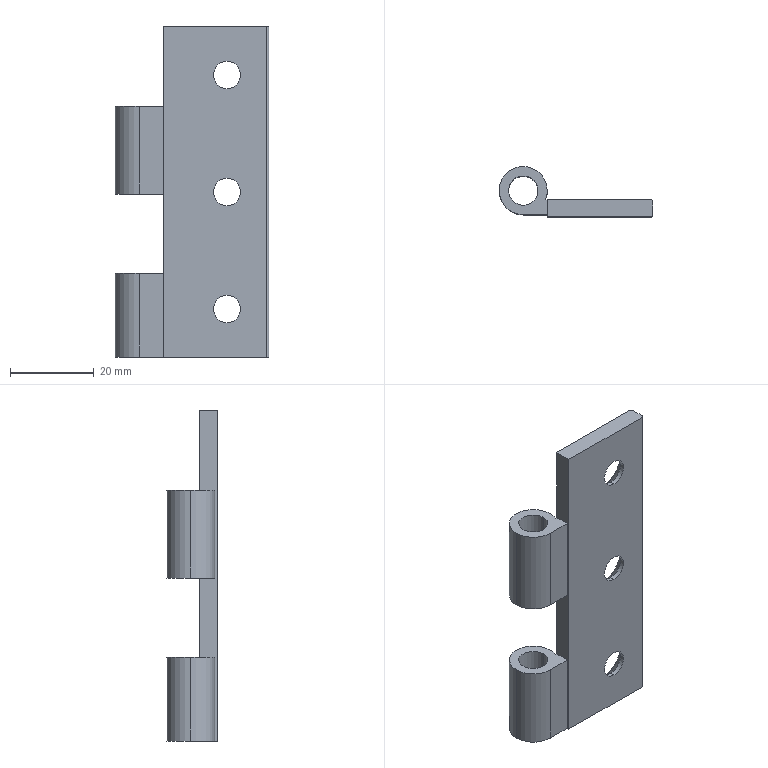Part | SolidWorks | features BaseBody 1 | 1 solid | 35 faces | box 36.75 x 12.05 x 79 mm | volume 10360 mm3 | cylinder 18 | plane 11 | cone 6 | commonest cylinder face diameters 6.5 x6 11.5 x6 7 x4 1 x2
STEP:
#1=CARTESIAN_POINT('',(21.,0.,-24.75));
#2=VERTEX_POINT('',#1);
#3=CARTESIAN_POINT('',(21.,0.,-31.25));
#4=VERTEX_POINT('',#3);
#5=CARTESIAN_POINT('',(21.,0.,-28.));
#6=DIRECTION('',(0.,-1.,0.));
#7=DIRECTION('',(0.,0.,1.));
#8=AXIS2_PLACEMENT_3D('',#5,#6,#7);
#9=CIRCLE('',#8,3.25);
#10=EDGE_CURVE('',#2,#4,#9,.T.);
#11=ORIENTED_EDGE('',*,*,#10,.T.);
#12=CARTESIAN_POINT('',(21.,1.1,-31.25));
#13=VERTEX_POINT('',#12);
#14=CARTESIAN_POINT('',(21.,0.,-31.25));
#15=DIRECTION('',(0.,1.,0.));
#16=VECTOR('',#15,1000.);
#17=LINE('',#14,#16);
#18=EDGE_CURVE('',#4,#13,#17,.T.);
#19=ORIENTED_EDGE('',*,*,#18,.T.);
#20=CARTESIAN_POINT('',(21.,1.1,-24.75));
#21=VERTEX_POINT('',#20);
#22=CARTESIAN_POINT('',(21.,1.1,-28.));
#23=DIRECTION('',(0.,-1.,0.));
#24=DIRECTION('',(0.,0.,1.));
#25=AXIS2_PLACEMENT_3D('',#22,#23,#24);
#26=CIRCLE('',#25,3.25);
#27=EDGE_CURVE('',#21,#13,#26,.T.);
#28=ORIENTED_EDGE('',*,*,#27,.F.);
#29=CARTESIAN_POINT('',(21.,0.,-24.75));
#30=DIRECTION('',(0.,1.,0.));
#31=VECTOR('',#30,1000.);
#32=LINE('',#29,#31);
#33=EDGE_CURVE('',#2,#21,#32,.T.);
#34=ORIENTED_EDGE('',*,*,#33,.F.);
#35=EDGE_LOOP('',(#11,#19,#28,#34));
#36=FACE_OUTER_BOUND('',#35,.T.);
#37=CARTESIAN_POINT('',(21.,0.,-28.));
#38=DIRECTION('',(0.,1.,0.));
#39=DIRECTION('',(0.,0.,1.));
#40=AXIS2_PLACEMENT_3D('',#37,#38,#39);
#41=CYLINDRICAL_SURFACE('',#40,3.25);
#42=ADVANCED_FACE('',(#36),#41,.F.);
#43=CARTESIAN_POINT('',(21.,0.,3.25));
#44=VERTEX_POINT('',#43);
#45=CARTESIAN_POINT('',(21.,0.,-3.25));
#46=VERTEX_POINT('',#45);
#47=CARTESIAN_POINT('',(21.,0.,0.));
#48=DIRECTION('',(0.,-1.,0.));
#49=DIRECTION('',(0.,0.,1.));
#50=AXIS2_PLACEMENT_3D('',#47,#48,#49);
#51=CIRCLE('',#50,3.25);
#52=EDGE_CURVE('',#44,#46,#51,.T.);
#53=ORIENTED_EDGE('',*,*,#52,.T.);
#54=CARTESIAN_POINT('',(21.,1.1,-3.25));
#55=VERTEX_POINT('',#54);
#56=CARTESIAN_POINT('',(21.,0.,-3.25));
#57=DIRECTION('',(0.,1.,0.));
#58=VECTOR('',#57,1000.);
#59=LINE('',#56,#58);
#60=EDGE_CURVE('',#46,#55,#59,.T.);
#61=ORIENTED_EDGE('',*,*,#60,.T.);
#62=CARTESIAN_POINT('',(21.,1.1,3.25));
#63=VERTEX_POINT('',#62);
#64=CARTESIAN_POINT('',(21.,1.1,0.));
#65=DIRECTION('',(0.,-1.,0.));
#66=DIRECTION('',(0.,0.,1.));
#67=AXIS2_PLACEMENT_3D('',#64,#65,#66);
#68=CIRCLE('',#67,3.25);
#69=EDGE_CURVE('',#63,#55,#68,.T.);
#70=ORIENTED_EDGE('',*,*,#69,.F.);
#71=CARTESIAN_POINT('',(21.,0.,3.25));
#72=DIRECTION('',(0.,1.,0.));
#73=VECTOR('',#72,1000.);
#74=LINE('',#71,#73);
#75=EDGE_CURVE('',#44,#63,#74,.T.);
#76=ORIENTED_EDGE('',*,*,#75,.F.);
#77=EDGE_LOOP('',(#53,#61,#70,#76));
#78=FACE_OUTER_BOUND('',#77,.T.);
#79=CARTESIAN_POINT('',(21.,0.,0.));
#80=DIRECTION('',(0.,1.,0.));
#81=DIRECTION('',(0.,0.,1.));
#82=AXIS2_PLACEMENT_3D('',#79,#80,#81);
#83=CYLINDRICAL_SURFACE('',#82,3.25);
#84=ADVANCED_FACE('',(#78),#83,.F.);
#85=CARTESIAN_POINT('',(21.,0.,31.25));
#86=VERTEX_POINT('',#85);
#87=CARTESIAN_POINT('',(21.,0.,24.75));
#88=VERTEX_POINT('',#87);
#89=CARTESIAN_POINT('',(21.,0.,28.));
#90=DIRECTION('',(0.,-1.,0.));
#91=DIRECTION('',(0.,0.,1.));
#92=AXIS2_PLACEMENT_3D('',#89,#90,#91);
#93=CIRCLE('',#92,3.25);
#94=EDGE_CURVE('',#86,#88,#93,.T.);
#95=ORIENTED_EDGE('',*,*,#94,.T.);
#96=CARTESIAN_POINT('',(21.,1.1,24.75));
#97=VERTEX_POINT('',#96);
#98=CARTESIAN_POINT('',(21.,0.,24.75));
#99=DIRECTION('',(0.,1.,0.));
#100=VECTOR('',#99,1000.);
#101=LINE('',#98,#100);
#102=EDGE_CURVE('',#88,#97,#101,.T.);
#103=ORIENTED_EDGE('',*,*,#102,.T.);
#104=CARTESIAN_POINT('',(21.,1.1,31.25));
#105=VERTEX_POINT('',#104);
#106=CARTESIAN_POINT('',(21.,1.1,28.));
#107=DIRECTION('',(0.,-1.,0.));
#108=DIRECTION('',(0.,0.,1.));
#109=AXIS2_PLACEMENT_3D('',#106,#107,#108);
#110=CIRCLE('',#109,3.25);
#111=EDGE_CURVE('',#105,#97,#110,.T.);
#112=ORIENTED_EDGE('',*,*,#111,.F.);
#113=CARTESIAN_POINT('',(21.,0.,31.25));
#114=DIRECTION('',(0.,1.,0.));
#115=VECTOR('',#114,1000.);
#116=LINE('',#113,#115);
#117=EDGE_CURVE('',#86,#105,#116,.T.);
#118=ORIENTED_EDGE('',*,*,#117,.F.);
#119=EDGE_LOOP('',(#95,#103,#112,#118));
#120=FACE_OUTER_BOUND('',#119,.T.);
#121=CARTESIAN_POINT('',(21.,0.,28.));
#122=DIRECTION('',(0.,1.,0.));
#123=DIRECTION('',(0.,0.,1.));
#124=AXIS2_PLACEMENT_3D('',#121,#122,#123);
#125=CYLINDRICAL_SURFACE('',#124,3.25);
#126=ADVANCED_FACE('',(#120),#125,.F.);
#127=CARTESIAN_POINT('',(5.75,6.3,-39.5));
#128=VERTEX_POINT('',#127);
#129=CARTESIAN_POINT('',(-5.75,6.3,-39.5));
#130=VERTEX_POINT('',#129);
#131=CARTESIAN_POINT('',(0.,6.3,-39.5));
#132=DIRECTION('',(0.,0.,1.));
#133=DIRECTION('',(1.,0.,0.));
#134=AXIS2_PLACEMENT_3D('',#131,#132,#133);
#135=CIRCLE('',#134,5.75);
#136=EDGE_CURVE('',#128,#130,#135,.T.);
#137=ORIENTED_EDGE('',*,*,#136,.T.);
#138=CARTESIAN_POINT('',(-5.75,6.3,-19.5));
#139=VERTEX_POINT('',#138);
#140=CARTESIAN_POINT('',(-5.75,6.3,39.5));
#141=DIRECTION('',(0.,0.,1.));
#142=VECTOR('',#141,1000.);
#143=LINE('',#140,#142);
#144=EDGE_CURVE('',#130,#139,#143,.T.);
#145=ORIENTED_EDGE('',*,*,#144,.T.);
#146=CARTESIAN_POINT('',(5.75,6.3,-19.5));
#147=VERTEX_POINT('',#146);
#148=CARTESIAN_POINT('',(0.,6.3,-19.5));
#149=DIRECTION('',(0.,0.,-1.));
#150=DIRECTION('',(1.,0.,0.));
#151=AXIS2_PLACEMENT_3D('',#148,#149,#150);
#152=CIRCLE('',#151,5.75);
#153=EDGE_CURVE('',#139,#147,#152,.T.);
#154=ORIENTED_EDGE('',*,*,#153,.T.);
#155=CARTESIAN_POINT('',(5.75,6.3,39.5));
#156=DIRECTION('',(0.,0.,1.));
#157=VECTOR('',#156,1000.);
#158=LINE('',#155,#157);
#159=EDGE_CURVE('',#128,#147,#158,.T.);
#160=ORIENTED_EDGE('',*,*,#159,.F.);
#161=EDGE_LOOP('',(#137,#145,#154,#160));
#162=FACE_OUTER_BOUND('',#161,.T.);
#163=CARTESIAN_POINT('',(0.,6.3,39.5));
#164=DIRECTION('',(0.,0.,1.));
#165=DIRECTION('',(1.,0.,0.));
#166=AXIS2_PLACEMENT_3D('',#163,#164,#165);
#167=CYLINDRICAL_SURFACE('',#166,5.75);
#168=ADVANCED_FACE('',(#162),#167,.T.);
#169=CARTESIAN_POINT('',(5.312,4.1,-39.5));
#170=VERTEX_POINT('',#169);
#171=CARTESIAN_POINT('',(0.,6.3,-39.5));
#172=DIRECTION('',(0.,0.,1.));
#173=DIRECTION('',(1.,0.,0.));
#174=AXIS2_PLACEMENT_3D('',#171,#172,#173);
#175=CIRCLE('',#174,5.75);
#176=EDGE_CURVE('',#170,#128,#175,.T.);
#177=ORIENTED_EDGE('',*,*,#176,.T.);
#178=ORIENTED_EDGE('',*,*,#159,.T.);
#179=CARTESIAN_POINT('',(5.312,4.1,-19.5));
#180=VERTEX_POINT('',#179);
#181=CARTESIAN_POINT('',(0.,6.3,-19.5));
#182=DIRECTION('',(0.,0.,-1.));
#183=DIRECTION('',(1.,0.,0.));
#184=AXIS2_PLACEMENT_3D('',#181,#182,#183);
#185=CIRCLE('',#184,5.75);
#186=EDGE_CURVE('',#147,#180,#185,.T.);
#187=ORIENTED_EDGE('',*,*,#186,.T.);
#188=CARTESIAN_POINT('',(5.312,4.1,39.5));
#189=DIRECTION('',(0.,0.,-1.));
#190=VECTOR('',#189,1000.);
#191=LINE('',#188,#190);
#192=EDGE_CURVE('',#180,#170,#191,.T.);
#193=ORIENTED_EDGE('',*,*,#192,.T.);
#194=EDGE_LOOP('',(#177,#178,#187,#193));
#195=FACE_OUTER_BOUND('',#194,.T.);
#196=CARTESIAN_POINT('',(0.,6.3,39.5));
#197=DIRECTION('',(0.,0.,1.));
#198=DIRECTION('',(1.,0.,0.));
#199=AXIS2_PLACEMENT_3D('',#196,#197,#198);
#200=CYLINDRICAL_SURFACE('',#199,5.75);
#201=ADVANCED_FACE('',(#195),#200,.T.);
#202=CARTESIAN_POINT('',(3.5,6.3,-39.5));
#203=VERTEX_POINT('',#202);
#204=CARTESIAN_POINT('',(-3.5,6.3,-39.5));
#205=VERTEX_POINT('',#204);
#206=CARTESIAN_POINT('',(0.,6.3,-39.5));
#207=DIRECTION('',(0.,0.,-1.));
#208=DIRECTION('',(1.,0.,0.));
#209=AXIS2_PLACEMENT_3D('',#206,#207,#208);
#210=CIRCLE('',#209,3.5);
#211=EDGE_CURVE('',#203,#205,#210,.T.);
#212=ORIENTED_EDGE('',*,*,#211,.T.);
#213=CARTESIAN_POINT('',(-3.5,6.3,-19.5));
#214=VERTEX_POINT('',#213);
#215=CARTESIAN_POINT('',(-3.5,6.3,39.5));
#216=DIRECTION('',(0.,0.,1.));
#217=VECTOR('',#216,1000.);
#218=LINE('',#215,#217);
#219=EDGE_CURVE('',#205,#214,#218,.T.);
#220=ORIENTED_EDGE('',*,*,#219,.T.);
#221=CARTESIAN_POINT('',(3.5,6.3,-19.5));
#222=VERTEX_POINT('',#221);
#223=CARTESIAN_POINT('',(0.,6.3,-19.5));
#224=DIRECTION('',(0.,0.,-1.));
#225=DIRECTION('',(1.,0.,0.));
#226=AXIS2_PLACEMENT_3D('',#223,#224,#225);
#227=CIRCLE('',#226,3.5);
#228=EDGE_CURVE('',#222,#214,#227,.T.);
#229=ORIENTED_EDGE('',*,*,#228,.F.);
#230=CARTESIAN_POINT('',(3.5,6.3,39.5));
#231=DIRECTION('',(0.,0.,1.));
#232=VECTOR('',#231,1000.);
#233=LINE('',#230,#232);
#234=EDGE_CURVE('',#203,#222,#233,.T.);
#235=ORIENTED_EDGE('',*,*,#234,.F.);
#236=EDGE_LOOP('',(#212,#220,#229,#235));
#237=FACE_OUTER_BOUND('',#236,.T.);
#238=CARTESIAN_POINT('',(0.,6.3,39.5));
#239=DIRECTION('',(0.,0.,1.));
#240=DIRECTION('',(1.,0.,0.));
#241=AXIS2_PLACEMENT_3D('',#238,#239,#240);
#242=CYLINDRICAL_SURFACE('',#241,3.5);
#243=ADVANCED_FACE('',(#237),#242,.F.);
#244=ORIENTED_EDGE('',*,*,#27,.T.);
#245=CARTESIAN_POINT('',(21.,4.1,-34.25));
#246=VERTEX_POINT('',#245);
#247=CARTESIAN_POINT('',(21.,4.1,-34.25));
#248=DIRECTION('',(0.,0.7071,-0.7071));
#249=VECTOR('',#248,1000.);
#250=LINE('',#247,#249);
#251=EDGE_CURVE('',#13,#246,#250,.T.);
#252=ORIENTED_EDGE('',*,*,#251,.T.);
#253=CARTESIAN_POINT('',(21.,4.1,-21.75));
#254=VERTEX_POINT('',#253);
#255=CARTESIAN_POINT('',(21.,4.1,-28.));
#256=DIRECTION('',(0.,1.,0.));
#257=DIRECTION('',(0.,0.,1.));
#258=AXIS2_PLACEMENT_3D('',#255,#256,#257);
#259=CIRCLE('',#258,6.25);
#260=EDGE_CURVE('',#246,#254,#259,.T.);
#261=ORIENTED_EDGE('',*,*,#260,.T.);
#262=CARTESIAN_POINT('',(21.,4.1,-21.75));
#263=DIRECTION('',(0.,0.7071,0.7071));
#264=VECTOR('',#263,1000.);
#265=LINE('',#262,#264);
#266=EDGE_CURVE('',#21,#254,#265,.T.);
#267=ORIENTED_EDGE('',*,*,#266,.F.);
#268=EDGE_LOOP('',(#244,#252,#261,#267));
#269=FACE_OUTER_BOUND('',#268,.T.);
#270=CARTESIAN_POINT('',(21.,4.1,-28.));
#271=DIRECTION('',(0.,1.,0.));
#272=DIRECTION('',(0.,0.,1.));
#273=AXIS2_PLACEMENT_3D('',#270,#271,#272);
#274=CONICAL_SURFACE('',#273,6.25,0.7854);
#275=ADVANCED_FACE('',(#269),#274,.F.);
#276=ORIENTED_EDGE('',*,*,#69,.T.);
#277=CARTESIAN_POINT('',(21.,4.1,-6.25));
#278=VERTEX_POINT('',#277);
#279=CARTESIAN_POINT('',(21.,4.1,-6.25));
#280=DIRECTION('',(0.,0.7071,-0.7071));
#281=VECTOR('',#280,1000.);
#282=LINE('',#279,#281);
#283=EDGE_CURVE('',#55,#278,#282,.T.);
#284=ORIENTED_EDGE('',*,*,#283,.T.);
#285=CARTESIAN_POINT('',(21.,4.1,6.25));
#286=VERTEX_POINT('',#285);
#287=CARTESIAN_POINT('',(21.,4.1,0.));
#288=DIRECTION('',(0.,1.,0.));
#289=DIRECTION('',(0.,0.,1.));
#290=AXIS2_PLACEMENT_3D('',#287,#288,#289);
#291=CIRCLE('',#290,6.25);
#292=EDGE_CURVE('',#278,#286,#291,.T.);
#293=ORIENTED_EDGE('',*,*,#292,.T.);
#294=CARTESIAN_POINT('',(21.,4.1,6.25));
#295=DIRECTION('',(0.,0.7071,0.7071));
#296=VECTOR('',#295,1000.);
#297=LINE('',#294,#296);
#298=EDGE_CURVE('',#63,#286,#297,.T.);
#299=ORIENTED_EDGE('',*,*,#298,.F.);
#300=EDGE_LOOP('',(#276,#284,#293,#299));
#301=FACE_OUTER_BOUND('',#300,.T.);
#302=CARTESIAN_POINT('',(21.,4.1,0.));
#303=DIRECTION('',(0.,1.,0.));
#304=DIRECTION('',(0.,0.,1.));
#305=AXIS2_PLACEMENT_3D('',#302,#303,#304);
#306=CONICAL_SURFACE('',#305,6.25,0.7854);
#307=ADVANCED_FACE('',(#301),#306,.F.);
#308=ORIENTED_EDGE('',*,*,#111,.T.);
#309=CARTESIAN_POINT('',(21.,4.1,21.75));
#310=VERTEX_POINT('',#309);
#311=CARTESIAN_POINT('',(21.,4.1,21.75));
#312=DIRECTION('',(0.,0.7071,-0.7071));
#313=VECTOR('',#312,1000.);
#314=LINE('',#311,#313);
#315=EDGE_CURVE('',#97,#310,#314,.T.);
#316=ORIENTED_EDGE('',*,*,#315,.T.);
#317=CARTESIAN_POINT('',(21.,4.1,34.25));
#318=VERTEX_POINT('',#317);
#319=CARTESIAN_POINT('',(21.,4.1,28.));
#320=DIRECTION('',(0.,1.,0.));
#321=DIRECTION('',(0.,0.,1.));
#322=AXIS2_PLACEMENT_3D('',#319,#320,#321);
#323=CIRCLE('',#322,6.25);
#324=EDGE_CURVE('',#310,#318,#323,.T.);
#325=ORIENTED_EDGE('',*,*,#324,.T.);
#326=CARTESIAN_POINT('',(21.,4.1,34.25));
#327=DIRECTION('',(0.,0.7071,0.7071));
#328=VECTOR('',#327,1000.);
#329=LINE('',#326,#328);
#330=EDGE_CURVE('',#105,#318,#329,.T.);
#331=ORIENTED_EDGE('',*,*,#330,.F.);
#332=EDGE_LOOP('',(#308,#316,#325,#331));
#333=FACE_OUTER_BOUND('',#332,.T.);
#334=CARTESIAN_POINT('',(21.,4.1,28.));
#335=DIRECTION('',(0.,1.,0.));
#336=DIRECTION('',(0.,0.,1.));
#337=AXIS2_PLACEMENT_3D('',#334,#335,#336);
#338=CONICAL_SURFACE('',#337,6.25,0.7854);
#339=ADVANCED_FACE('',(#333),#338,.F.);
#340=CARTESIAN_POINT('',(-5.75,6.3,-0.5));
#341=VERTEX_POINT('',#340);
#342=CARTESIAN_POINT('',(5.75,6.3,-0.5));
#343=VERTEX_POINT('',#342);
#344=CARTESIAN_POINT('',(0.,6.3,-0.5));
#345=DIRECTION('',(0.,0.,-1.));
#346=DIRECTION('',(1.,0.,0.));
#347=AXIS2_PLACEMENT_3D('',#344,#345,#346);
#348=CIRCLE('',#347,5.75);
#349=EDGE_CURVE('',#341,#343,#348,.T.);
#350=ORIENTED_EDGE('',*,*,#349,.F.);
#351=CARTESIAN_POINT('',(-5.75,6.3,20.5));
#352=VERTEX_POINT('',#351);
#353=CARTESIAN_POINT('',(-5.75,6.3,39.5));
#354=DIRECTION('',(0.,0.,1.));
#355=VECTOR('',#354,1000.);
#356=LINE('',#353,#355);
#357=EDGE_CURVE('',#341,#352,#356,.T.);
#358=ORIENTED_EDGE('',*,*,#357,.T.);
#359=CARTESIAN_POINT('',(5.75,6.3,20.5));
#360=VERTEX_POINT('',#359);
#361=CARTESIAN_POINT('',(0.,6.3,20.5));
#362=DIRECTION('',(0.,0.,1.));
#363=DIRECTION('',(1.,0.,0.));
#364=AXIS2_PLACEMENT_3D('',#361,#362,#363);
#365=CIRCLE('',#364,5.75);
#366=EDGE_CURVE('',#360,#352,#365,.T.);
#367=ORIENTED_EDGE('',*,*,#366,.F.);
#368=CARTESIAN_POINT('',(5.75,6.3,39.5));
#369=DIRECTION('',(0.,0.,1.));
#370=VECTOR('',#369,1000.);
#371=LINE('',#368,#370);
#372=EDGE_CURVE('',#343,#360,#371,.T.);
#373=ORIENTED_EDGE('',*,*,#372,.F.);
#374=EDGE_LOOP('',(#350,#358,#367,#373));
#375=FACE_OUTER_BOUND('',#374,.T.);
#376=CARTESIAN_POINT('',(0.,6.3,39.5));
#377=DIRECTION('',(0.,0.,1.));
#378=DIRECTION('',(1.,0.,0.));
#379=AXIS2_PLACEMENT_3D('',#376,#377,#378);
#380=CYLINDRICAL_SURFACE('',#379,5.75);
#381=ADVANCED_FACE('',(#375),#380,.T.);
#382=CARTESIAN_POINT('',(5.312,4.1,-0.5));
#383=VERTEX_POINT('',#382);
#384=CARTESIAN_POINT('',(0.,6.3,-0.5));
#385=DIRECTION('',(0.,0.,-1.));
#386=DIRECTION('',(1.,0.,0.));
#387=AXIS2_PLACEMENT_3D('',#384,#385,#386);
#388=CIRCLE('',#387,5.75);
#389=EDGE_CURVE('',#343,#383,#388,.T.);
#390=ORIENTED_EDGE('',*,*,#389,.F.);
#391=ORIENTED_EDGE('',*,*,#372,.T.);
#392=CARTESIAN_POINT('',(5.312,4.1,20.5));
#393=VERTEX_POINT('',#392);
#394=CARTESIAN_POINT('',(0.,6.3,20.5));
#395=DIRECTION('',(0.,0.,1.));
#396=DIRECTION('',(1.,0.,0.));
#397=AXIS2_PLACEMENT_3D('',#394,#395,#396);
#398=CIRCLE('',#397,5.75);
#399=EDGE_CURVE('',#393,#360,#398,.T.);
#400=ORIENTED_EDGE('',*,*,#399,.F.);
#401=CARTESIAN_POINT('',(5.312,4.1,39.5));
#402=DIRECTION('',(0.,0.,-1.));
#403=VECTOR('',#402,1000.);
#404=LINE('',#401,#403);
#405=EDGE_CURVE('',#393,#383,#404,.T.);
#406=ORIENTED_EDGE('',*,*,#405,.T.);
#407=EDGE_LOOP('',(#390,#391,#400,#406));
#408=FACE_OUTER_BOUND('',#407,.T.);
#409=CARTESIAN_POINT('',(0.,6.3,39.5));
#410=DIRECTION('',(0.,0.,1.));
#411=DIRECTION('',(1.,0.,0.));
#412=AXIS2_PLACEMENT_3D('',#409,#410,#411);
#413=CYLINDRICAL_SURFACE('',#412,5.75);
#414=ADVANCED_FACE('',(#408),#413,.T.);
#415=CARTESIAN_POINT('',(-3.5,6.3,-0.5));
#416=VERTEX_POINT('',#415);
#417=CARTESIAN_POINT('',(3.5,6.3,-0.5));
#418=VERTEX_POINT('',#417);
#419=CARTESIAN_POINT('',(0.,6.3,-0.5));
#420=DIRECTION('',(0.,0.,1.));
#421=DIRECTION('',(1.,0.,0.));
#422=AXIS2_PLACEMENT_3D('',#419,#420,#421);
#423=CIRCLE('',#422,3.5);
#424=EDGE_CURVE('',#416,#418,#423,.T.);
#425=ORIENTED_EDGE('',*,*,#424,.F.);
#426=CARTESIAN_POINT('',(-3.5,6.3,20.5));
#427=VERTEX_POINT('',#426);
#428=CARTESIAN_POINT('',(-3.5,6.3,39.5));
#429=DIRECTION('',(0.,0.,1.));
#430=VECTOR('',#429,1000.);
#431=LINE('',#428,#430);
#432=EDGE_CURVE('',#416,#427,#431,.T.);
#433=ORIENTED_EDGE('',*,*,#432,.T.);
#434=CARTESIAN_POINT('',(3.5,6.3,20.5));
#435=VERTEX_POINT('',#434);
#436=CARTESIAN_POINT('',(0.,6.3,20.5));
#437=DIRECTION('',(0.,0.,-1.));
#438=DIRECTION('',(1.,0.,0.));
#439=AXIS2_PLACEMENT_3D('',#436,#437,#438);
#440=CIRCLE('',#439,3.5);
#441=EDGE_CURVE('',#435,#427,#440,.T.);
#442=ORIENTED_EDGE('',*,*,#441,.F.);
#443=CARTESIAN_POINT('',(3.5,6.3,39.5));
#444=DIRECTION('',(0.,0.,1.));
#445=VECTOR('',#444,1000.);
#446=LINE('',#443,#445);
#447=EDGE_CURVE('',#418,#435,#446,.T.);
#448=ORIENTED_EDGE('',*,*,#447,.F.);
#449=EDGE_LOOP('',(#425,#433,#442,#448));
#450=FACE_OUTER_BOUND('',#449,.T.);
#451=CARTESIAN_POINT('',(0.,6.3,39.5));
#452=DIRECTION('',(0.,0.,1.));
#453=DIRECTION('',(1.,0.,0.));
#454=AXIS2_PLACEMENT_3D('',#451,#452,#453);
#455=CYLINDRICAL_SURFACE('',#454,3.5);
#456=ADVANCED_FACE('',(#450),#455,.F.);
#457=CARTESIAN_POINT('',(30.5,0.,39.5));
#458=VERTEX_POINT('',#457);
#459=CARTESIAN_POINT('',(30.5,0.,-39.5));
#460=VERTEX_POINT('',#459);
#461=CARTESIAN_POINT('',(30.5,0.,39.5));
#462=DIRECTION('',(0.,0.,-1.));
#463=VECTOR('',#462,1000.);
#464=LINE('',#461,#463);
#465=EDGE_CURVE('',#458,#460,#464,.T.);
#466=ORIENTED_EDGE('',*,*,#465,.F.);
#467=CARTESIAN_POINT('',(5.75,0.,39.5));
#468=VERTEX_POINT('',#467);
#469=CARTESIAN_POINT('',(5.75,0.,39.5));
#470=DIRECTION('',(1.,0.,0.));
#471=VECTOR('',#470,1000.);
#472=LINE('',#469,#471);
#473=EDGE_CURVE('',#468,#458,#472,.T.);
#474=ORIENTED_EDGE('',*,*,#473,.F.);
#475=CARTESIAN_POINT('',(5.75,0.,-39.5));
#476=VERTEX_POINT('',#475);
#477=CARTESIAN_POINT('',(5.75,0.,39.5));
#478=DIRECTION('',(0.,0.,1.));
#479=VECTOR('',#478,1000.);
#480=LINE('',#477,#479);
#481=EDGE_CURVE('',#476,#468,#480,.T.);
#482=ORIENTED_EDGE('',*,*,#481,.F.);
#483=CARTESIAN_POINT('',(5.75,0.,-39.5));
#484=DIRECTION('',(-1.,0.,0.));
#485=VECTOR('',#484,1000.);
#486=LINE('',#483,#485);
#487=EDGE_CURVE('',#460,#476,#486,.T.);
#488=ORIENTED_EDGE('',*,*,#487,.F.);
#489=EDGE_LOOP('',(#466,#474,#482,#488));
#490=FACE_OUTER_BOUND('',#489,.T.);
#491=ORIENTED_EDGE('',*,*,#10,.F.);
#492=CARTESIAN_POINT('',(21.,0.,-28.));
#493=DIRECTION('',(0.,-1.,0.));
#494=DIRECTION('',(0.,0.,1.));
#495=AXIS2_PLACEMENT_3D('',#492,#493,#494);
#496=CIRCLE('',#495,3.25);
#497=EDGE_CURVE('',#4,#2,#496,.T.);
#498=ORIENTED_EDGE('',*,*,#497,.F.);
#499=EDGE_LOOP('',(#491,#498));
#500=FACE_BOUND('',#499,.T.);
#501=ORIENTED_EDGE('',*,*,#52,.F.);
#502=CARTESIAN_POINT('',(21.,0.,0.));
#503=DIRECTION('',(0.,-1.,0.));
#504=DIRECTION('',(0.,0.,1.));
#505=AXIS2_PLACEMENT_3D('',#502,#503,#504);
#506=CIRCLE('',#505,3.25);
#507=EDGE_CURVE('',#46,#44,#506,.T.);
#508=ORIENTED_EDGE('',*,*,#507,.F.);
#509=EDGE_LOOP('',(#501,#508));
#510=FACE_BOUND('',#509,.T.);
#511=ORIENTED_EDGE('',*,*,#94,.F.);
#512=CARTESIAN_POINT('',(21.,0.,28.));
#513=DIRECTION('',(0.,-1.,0.));
#514=DIRECTION('',(0.,0.,1.));
#515=AXIS2_PLACEMENT_3D('',#512,#513,#514);
#516=CIRCLE('',#515,3.25);
#517=EDGE_CURVE('',#88,#86,#516,.T.);
#518=ORIENTED_EDGE('',*,*,#517,.F.);
#519=EDGE_LOOP('',(#511,#518));
#520=FACE_BOUND('',#519,.T.);
#521=CARTESIAN_POINT('',(5.75,0.,39.5));
#522=DIRECTION('',(0.,1.,0.));
#523=DIRECTION('',(0.,0.,1.));
#524=AXIS2_PLACEMENT_3D('',#521,#522,#523);
#525=PLANE('',#524);
#526=ADVANCED_FACE('',(#490,#500,#510,#520),#525,.F.);
#527=CARTESIAN_POINT('',(31.,3.6,-39.5));
#528=VERTEX_POINT('',#527);
#529=CARTESIAN_POINT('',(30.5,4.1,-39.5));
#530=VERTEX_POINT('',#529);
#531=CARTESIAN_POINT('',(30.5,3.6,-39.5));
#532=DIRECTION('',(0.,0.,1.));
#533=DIRECTION('',(1.,0.,0.));
#534=AXIS2_PLACEMENT_3D('',#531,#532,#533);
#535=CIRCLE('',#534,0.5);
#536=EDGE_CURVE('',#528,#530,#535,.T.);
#537=ORIENTED_EDGE('',*,*,#536,.F.);
#538=CARTESIAN_POINT('',(31.,0.5,-39.5));
#539=VERTEX_POINT('',#538);
#540=CARTESIAN_POINT('',(31.,6.3,-39.5));
#541=DIRECTION('',(0.,1.,0.));
#542=VECTOR('',#541,1000.);
#543=LINE('',#540,#542);
#544=EDGE_CURVE('',#539,#528,#543,.T.);
#545=ORIENTED_EDGE('',*,*,#544,.F.);
#546=CARTESIAN_POINT('',(30.5,0.5,-39.5));
#547=DIRECTION('',(0.,0.,1.));
#548=DIRECTION('',(1.,0.,0.));
#549=AXIS2_PLACEMENT_3D('',#546,#547,#548);
#550=CIRCLE('',#549,0.5);
#551=EDGE_CURVE('',#460,#539,#550,.T.);
#552=ORIENTED_EDGE('',*,*,#551,.F.);
#553=ORIENTED_EDGE('',*,*,#487,.T.);
#554=CARTESIAN_POINT('',(5.75,0.55,-39.5));
#555=VERTEX_POINT('',#554);
#556=CARTESIAN_POINT('',(5.75,6.3,-39.5));
#557=DIRECTION('',(0.,-1.,0.));
#558=VECTOR('',#557,1000.);
#559=LINE('',#556,#558);
#560=EDGE_CURVE('',#555,#476,#559,.T.);
#561=ORIENTED_EDGE('',*,*,#560,.F.);
#562=CARTESIAN_POINT('',(0.,0.55,-39.5));
#563=VERTEX_POINT('',#562);
#564=CARTESIAN_POINT('',(0.,0.55,-39.5));
#565=DIRECTION('',(1.,0.,0.));
#566=VECTOR('',#565,1000.);
#567=LINE('',#564,#566);
#568=EDGE_CURVE('',#563,#555,#567,.T.);
#569=ORIENTED_EDGE('',*,*,#568,.F.);
#570=CARTESIAN_POINT('',(0.,6.3,-39.5));
#571=DIRECTION('',(0.,0.,1.));
#572=DIRECTION('',(1.,0.,0.));
#573=AXIS2_PLACEMENT_3D('',#570,#571,#572);
#574=CIRCLE('',#573,5.75);
#575=EDGE_CURVE('',#130,#563,#574,.T.);
#576=ORIENTED_EDGE('',*,*,#575,.F.);
#577=ORIENTED_EDGE('',*,*,#136,.F.);
#578=ORIENTED_EDGE('',*,*,#176,.F.);
#579=CARTESIAN_POINT('',(0.,4.1,-39.5));
#580=DIRECTION('',(-1.,0.,0.));
#581=VECTOR('',#580,1000.);
#582=LINE('',#579,#581);
#583=EDGE_CURVE('',#530,#170,#582,.T.);
#584=ORIENTED_EDGE('',*,*,#583,.F.);
#585=EDGE_LOOP('',(#537,#545,#552,#553,#561,#569,#576,#577,#578,#584));
#586=FACE_OUTER_BOUND('',#585,.T.);
#587=ORIENTED_EDGE('',*,*,#211,.F.);
#588=CARTESIAN_POINT('',(0.,6.3,-39.5));
#589=DIRECTION('',(0.,0.,-1.));
#590=DIRECTION('',(1.,0.,0.));
#591=AXIS2_PLACEMENT_3D('',#588,#589,#590);
#592=CIRCLE('',#591,3.5);
#593=EDGE_CURVE('',#205,#203,#592,.T.);
#594=ORIENTED_EDGE('',*,*,#593,.F.);
#595=EDGE_LOOP('',(#587,#594));
#596=FACE_BOUND('',#595,.T.);
#597=CARTESIAN_POINT('',(0.,6.3,-39.5));
#598=DIRECTION('',(0.,0.,1.));
#599=DIRECTION('',(1.,0.,0.));
#600=AXIS2_PLACEMENT_3D('',#597,#598,#599);
#601=PLANE('',#600);
#602=ADVANCED_FACE('',(#586,#596),#601,.F.);
#603=CARTESIAN_POINT('',(31.,0.5,39.5));
#604=VERTEX_POINT('',#603);
#605=CARTESIAN_POINT('',(30.5,0.5,39.5));
#606=DIRECTION('',(0.,0.,-1.));
#607=DIRECTION('',(1.,0.,0.));
#608=AXIS2_PLACEMENT_3D('',#605,#606,#607);
#609=CIRCLE('',#608,0.5);
#610=EDGE_CURVE('',#604,#458,#609,.T.);
#611=ORIENTED_EDGE('',*,*,#610,.T.);
#612=ORIENTED_EDGE('',*,*,#465,.T.);
#613=ORIENTED_EDGE('',*,*,#551,.T.);
#614=CARTESIAN_POINT('',(31.,0.5,39.5));
#615=DIRECTION('',(0.,0.,1.));
#616=VECTOR('',#615,1000.);
#617=LINE('',#614,#616);
#618=EDGE_CURVE('',#539,#604,#617,.T.);
#619=ORIENTED_EDGE('',*,*,#618,.T.);
#620=EDGE_LOOP('',(#611,#612,#613,#619));
#621=FACE_OUTER_BOUND('',#620,.T.);
#622=CARTESIAN_POINT('',(30.5,0.5,39.5));
#623=DIRECTION('',(0.,0.,1.));
#624=DIRECTION('',(1.,0.,0.));
#625=AXIS2_PLACEMENT_3D('',#622,#623,#624);
#626=CYLINDRICAL_SURFACE('',#625,0.5);
#627=ADVANCED_FACE('',(#621),#626,.T.);
#628=CARTESIAN_POINT('',(31.,3.6,39.5));
#629=VERTEX_POINT('',#628);
#630=CARTESIAN_POINT('',(31.,6.3,39.5));
#631=DIRECTION('',(0.,1.,0.));
#632=VECTOR('',#631,1000.);
#633=LINE('',#630,#632);
#634=EDGE_CURVE('',#604,#629,#633,.T.);
#635=ORIENTED_EDGE('',*,*,#634,.T.);
#636=CARTESIAN_POINT('',(30.5,4.1,39.5));
#637=VERTEX_POINT('',#636);
#638=CARTESIAN_POINT('',(30.5,3.6,39.5));
#639=DIRECTION('',(0.,0.,-1.));
#640=DIRECTION('',(1.,0.,0.));
#641=AXIS2_PLACEMENT_3D('',#638,#639,#640);
#642=CIRCLE('',#641,0.5);
#643=EDGE_CURVE('',#637,#629,#642,.T.);
#644=ORIENTED_EDGE('',*,*,#643,.F.);
#645=CARTESIAN_POINT('',(5.75,4.1,39.5));
#646=VERTEX_POINT('',#645);
#647=CARTESIAN_POINT('',(0.,4.1,39.5));
#648=DIRECTION('',(-1.,0.,0.));
#649=VECTOR('',#648,1000.);
#650=LINE('',#647,#649);
#651=EDGE_CURVE('',#637,#646,#650,.T.);
#652=ORIENTED_EDGE('',*,*,#651,.T.);
#653=CARTESIAN_POINT('',(5.75,6.3,39.5));
#654=DIRECTION('',(0.,-1.,0.));
#655=VECTOR('',#654,1000.);
#656=LINE('',#653,#655);
#657=EDGE_CURVE('',#646,#468,#656,.T.);
#658=ORIENTED_EDGE('',*,*,#657,.T.);
#659=ORIENTED_EDGE('',*,*,#473,.T.);
#660=ORIENTED_EDGE('',*,*,#610,.F.);
#661=EDGE_LOOP('',(#635,#644,#652,#658,#659,#660));
#662=FACE_OUTER_BOUND('',#661,.T.);
#663=CARTESIAN_POINT('',(0.,6.3,39.5));
#664=DIRECTION('',(0.,0.,1.));
#665=DIRECTION('',(1.,0.,0.));
#666=AXIS2_PLACEMENT_3D('',#663,#664,#665);
#667=PLANE('',#666);
#668=ADVANCED_FACE('',(#662),#667,.T.);
#669=CARTESIAN_POINT('',(5.75,4.1,-0.5));
#670=VERTEX_POINT('',#669);
#671=CARTESIAN_POINT('',(5.75,0.55,-0.5));
#672=VERTEX_POINT('',#671);
#673=CARTESIAN_POINT('',(5.75,0.55,-0.5));
#674=DIRECTION('',(0.,-1.,0.));
#675=VECTOR('',#674,1000.);
#676=LINE('',#673,#675);
#677=EDGE_CURVE('',#670,#672,#676,.T.);
#678=ORIENTED_EDGE('',*,*,#677,.F.);
#679=CARTESIAN_POINT('',(5.75,4.1,-19.5));
#680=VERTEX_POINT('',#679);
#681=CARTESIAN_POINT('',(5.75,4.1,39.5));
#682=DIRECTION('',(0.,0.,1.));
#683=VECTOR('',#682,1000.);
#684=LINE('',#681,#683);
#685=EDGE_CURVE('',#680,#670,#684,.T.);
#686=ORIENTED_EDGE('',*,*,#685,.F.);
#687=CARTESIAN_POINT('',(5.75,0.55,-19.5));
#688=VERTEX_POINT('',#687);
#689=CARTESIAN_POINT('',(5.75,0.55,-19.5));
#690=DIRECTION('',(0.,1.,0.));
#691=VECTOR('',#690,1000.);
#692=LINE('',#689,#691);
#693=EDGE_CURVE('',#688,#680,#692,.T.);
#694=ORIENTED_EDGE('',*,*,#693,.F.);
#695=CARTESIAN_POINT('',(5.75,0.55,39.5));
#696=DIRECTION('',(0.,0.,1.));
#697=VECTOR('',#696,1000.);
#698=LINE('',#695,#697);
#699=EDGE_CURVE('',#555,#688,#698,.T.);
#700=ORIENTED_EDGE('',*,*,#699,.F.);
#701=ORIENTED_EDGE('',*,*,#560,.T.);
#702=ORIENTED_EDGE('',*,*,#481,.T.);
#703=ORIENTED_EDGE('',*,*,#657,.F.);
#704=CARTESIAN_POINT('',(5.75,4.1,20.5));
#705=VERTEX_POINT('',#704);
#706=CARTESIAN_POINT('',(5.75,4.1,39.5));
#707=DIRECTION('',(0.,0.,1.));
#708=VECTOR('',#707,1000.);
#709=LINE('',#706,#708);
#710=EDGE_CURVE('',#705,#646,#709,.T.);
#711=ORIENTED_EDGE('',*,*,#710,.F.);
#712=CARTESIAN_POINT('',(5.75,0.55,20.5));
#713=VERTEX_POINT('',#712);
#714=CARTESIAN_POINT('',(5.75,0.55,20.5));
#715=DIRECTION('',(0.,1.,0.));
#716=VECTOR('',#715,1000.);
#717=LINE('',#714,#716);
#718=EDGE_CURVE('',#713,#705,#717,.T.);
#719=ORIENTED_EDGE('',*,*,#718,.F.);
#720=CARTESIAN_POINT('',(5.75,0.55,39.5));
#721=DIRECTION('',(0.,0.,1.));
#722=VECTOR('',#721,1000.);
#723=LINE('',#720,#722);
#724=EDGE_CURVE('',#672,#713,#723,.T.);
#725=ORIENTED_EDGE('',*,*,#724,.F.);
#726=EDGE_LOOP('',(#678,#686,#694,#700,#701,#702,#703,#711,#719,#725));
#727=FACE_OUTER_BOUND('',#726,.T.);
#728=CARTESIAN_POINT('',(5.75,0.55,39.5));
#729=DIRECTION('',(1.,0.,0.));
#730=DIRECTION('',(0.,1.,0.));
#731=AXIS2_PLACEMENT_3D('',#728,#729,#730);
#732=PLANE('',#731);
#733=ADVANCED_FACE('',(#727),#732,.F.);
#734=ORIENTED_EDGE('',*,*,#18,.F.);
#735=ORIENTED_EDGE('',*,*,#497,.T.);
#736=ORIENTED_EDGE('',*,*,#33,.T.);
#737=CARTESIAN_POINT('',(21.,1.1,-28.));
#738=DIRECTION('',(0.,-1.,0.));
#739=DIRECTION('',(0.,0.,1.));
#740=AXIS2_PLACEMENT_3D('',#737,#738,#739);
#741=CIRCLE('',#740,3.25);
#742=EDGE_CURVE('',#13,#21,#741,.T.);
#743=ORIENTED_EDGE('',*,*,#742,.F.);
#744=EDGE_LOOP('',(#734,#735,#736,#743));
#745=FACE_OUTER_BOUND('',#744,.T.);
#746=CARTESIAN_POINT('',(21.,0.,-28.));
#747=DIRECTION('',(0.,1.,0.));
#748=DIRECTION('',(0.,0.,1.));
#749=AXIS2_PLACEMENT_3D('',#746,#747,#748);
#750=CYLINDRICAL_SURFACE('',#749,3.25);
#751=ADVANCED_FACE('',(#745),#750,.F.);
#752=ORIENTED_EDGE('',*,*,#60,.F.);
#753=ORIENTED_EDGE('',*,*,#507,.T.);
#754=ORIENTED_EDGE('',*,*,#75,.T.);
#755=CARTESIAN_POINT('',(21.,1.1,0.));
#756=DIRECTION('',(0.,-1.,0.));
#757=DIRECTION('',(0.,0.,1.));
#758=AXIS2_PLACEMENT_3D('',#755,#756,#757);
#759=CIRCLE('',#758,3.25);
#760=EDGE_CURVE('',#55,#63,#759,.T.);
#761=ORIENTED_EDGE('',*,*,#760,.F.);
#762=EDGE_LOOP('',(#752,#753,#754,#761));
#763=FACE_OUTER_BOUND('',#762,.T.);
#764=CARTESIAN_POINT('',(21.,0.,0.));
#765=DIRECTION('',(0.,1.,0.));
#766=DIRECTION('',(0.,0.,1.));
#767=AXIS2_PLACEMENT_3D('',#764,#765,#766);
#768=CYLINDRICAL_SURFACE('',#767,3.25);
#769=ADVANCED_FACE('',(#763),#768,.F.);
#770=ORIENTED_EDGE('',*,*,#102,.F.);
#771=ORIENTED_EDGE('',*,*,#517,.T.);
#772=ORIENTED_EDGE('',*,*,#117,.T.);
#773=CARTESIAN_POINT('',(21.,1.1,28.));
#774=DIRECTION('',(0.,-1.,0.));
#775=DIRECTION('',(0.,0.,1.));
#776=AXIS2_PLACEMENT_3D('',#773,#774,#775);
#777=CIRCLE('',#776,3.25);
#778=EDGE_CURVE('',#97,#105,#777,.T.);
#779=ORIENTED_EDGE('',*,*,#778,.F.);
#780=EDGE_LOOP('',(#770,#771,#772,#779));
#781=FACE_OUTER_BOUND('',#780,.T.);
#782=CARTESIAN_POINT('',(21.,0.,28.));
#783=DIRECTION('',(0.,1.,0.));
#784=DIRECTION('',(0.,0.,1.));
#785=AXIS2_PLACEMENT_3D('',#782,#783,#784);
#786=CYLINDRICAL_SURFACE('',#785,3.25);
#787=ADVANCED_FACE('',(#781),#786,.F.);
#788=ORIENTED_EDGE('',*,*,#651,.F.);
#789=CARTESIAN_POINT('',(30.5,4.1,39.5));
#790=DIRECTION('',(0.,0.,1.));
#791=VECTOR('',#790,1000.);
#792=LINE('',#789,#791);
#793=EDGE_CURVE('',#530,#637,#792,.T.);
#794=ORIENTED_EDGE('',*,*,#793,.F.);
#795=ORIENTED_EDGE('',*,*,#583,.T.);
#796=ORIENTED_EDGE('',*,*,#192,.F.);
#797=CARTESIAN_POINT('',(30.5,4.1,-19.5));
#798=DIRECTION('',(-1.,0.,0.));
#799=VECTOR('',#798,1000.);
#800=LINE('',#797,#799);
#801=EDGE_CURVE('',#680,#180,#800,.T.);
#802=ORIENTED_EDGE('',*,*,#801,.F.);
#803=ORIENTED_EDGE('',*,*,#685,.T.);
#804=CARTESIAN_POINT('',(30.5,4.1,-0.5));
#805=DIRECTION('',(1.,0.,0.));
#806=VECTOR('',#805,1000.);
#807=LINE('',#804,#806);
#808=EDGE_CURVE('',#383,#670,#807,.T.);
#809=ORIENTED_EDGE('',*,*,#808,.F.);
#810=ORIENTED_EDGE('',*,*,#405,.F.);
#811=CARTESIAN_POINT('',(30.5,4.1,20.5));
#812=DIRECTION('',(-1.,0.,0.));
#813=VECTOR('',#812,1000.);
#814=LINE('',#811,#813);
#815=EDGE_CURVE('',#705,#393,#814,.T.);
#816=ORIENTED_EDGE('',*,*,#815,.F.);
#817=ORIENTED_EDGE('',*,*,#710,.T.);
#818=EDGE_LOOP('',(#788,#794,#795,#796,#802,#803,#809,#810,#816,#817));
#819=FACE_OUTER_BOUND('',#818,.T.);
#820=CARTESIAN_POINT('',(21.,4.1,-28.));
#821=DIRECTION('',(0.,1.,0.));
#822=DIRECTION('',(0.,0.,1.));
#823=AXIS2_PLACEMENT_3D('',#820,#821,#822);
#824=CIRCLE('',#823,6.25);
#825=EDGE_CURVE('',#254,#246,#824,.T.);
#826=ORIENTED_EDGE('',*,*,#825,.F.);
#827=ORIENTED_EDGE('',*,*,#260,.F.);
#828=EDGE_LOOP('',(#826,#827));
#829=FACE_BOUND('',#828,.T.);
#830=CARTESIAN_POINT('',(21.,4.1,0.));
#831=DIRECTION('',(0.,1.,0.));
#832=DIRECTION('',(0.,0.,1.));
#833=AXIS2_PLACEMENT_3D('',#830,#831,#832);
#834=CIRCLE('',#833,6.25);
#835=EDGE_CURVE('',#286,#278,#834,.T.);
#836=ORIENTED_EDGE('',*,*,#835,.F.);
#837=ORIENTED_EDGE('',*,*,#292,.F.);
#838=EDGE_LOOP('',(#836,#837));
#839=FACE_BOUND('',#838,.T.);
#840=CARTESIAN_POINT('',(21.,4.1,28.));
#841=DIRECTION('',(0.,1.,0.));
#842=DIRECTION('',(0.,0.,1.));
#843=AXIS2_PLACEMENT_3D('',#840,#841,#842);
#844=CIRCLE('',#843,6.25);
#845=EDGE_CURVE('',#318,#310,#844,.T.);
#846=ORIENTED_EDGE('',*,*,#845,.F.);
#847=ORIENTED_EDGE('',*,*,#324,.F.);
#848=EDGE_LOOP('',(#846,#847));
#849=FACE_BOUND('',#848,.T.);
#850=CARTESIAN_POINT('',(30.5,4.1,39.5));
#851=DIRECTION('',(0.,-1.,0.));
#852=DIRECTION('',(0.,0.,-1.));
#853=AXIS2_PLACEMENT_3D('',#850,#851,#852);
#854=PLANE('',#853);
#855=ADVANCED_FACE('',(#819,#829,#839,#849),#854,.F.);
#856=CARTESIAN_POINT('',(31.,3.6,39.5));
#857=DIRECTION('',(0.,0.,-1.));
#858=VECTOR('',#857,1000.);
#859=LINE('',#856,#858);
#860=EDGE_CURVE('',#629,#528,#859,.T.);
#861=ORIENTED_EDGE('',*,*,#860,.F.);
#862=ORIENTED_EDGE('',*,*,#634,.F.);
#863=ORIENTED_EDGE('',*,*,#618,.F.);
#864=ORIENTED_EDGE('',*,*,#544,.T.);
#865=EDGE_LOOP('',(#861,#862,#863,#864));
#866=FACE_OUTER_BOUND('',#865,.T.);
#867=CARTESIAN_POINT('',(31.,0.5,39.5));
#868=DIRECTION('',(-1.,0.,0.));
#869=DIRECTION('',(0.,0.,1.));
#870=AXIS2_PLACEMENT_3D('',#867,#868,#869);
#871=PLANE('',#870);
#872=ADVANCED_FACE('',(#866),#871,.F.);
#873=CARTESIAN_POINT('',(0.,0.55,-19.5));
#874=VERTEX_POINT('',#873);
#875=CARTESIAN_POINT('',(0.,0.55,39.5));
#876=DIRECTION('',(0.,0.,1.));
#877=VECTOR('',#876,1000.);
#878=LINE('',#875,#877);
#879=EDGE_CURVE('',#563,#874,#878,.T.);
#880=ORIENTED_EDGE('',*,*,#879,.F.);
#881=ORIENTED_EDGE('',*,*,#568,.T.);
#882=ORIENTED_EDGE('',*,*,#699,.T.);
#883=CARTESIAN_POINT('',(0.,0.55,-19.5));
#884=DIRECTION('',(1.,0.,0.));
#885=VECTOR('',#884,1000.);
#886=LINE('',#883,#885);
#887=EDGE_CURVE('',#874,#688,#886,.T.);
#888=ORIENTED_EDGE('',*,*,#887,.F.);
#889=EDGE_LOOP('',(#880,#881,#882,#888));
#890=FACE_OUTER_BOUND('',#889,.T.);
#891=CARTESIAN_POINT('',(0.,0.55,39.5));
#892=DIRECTION('',(0.,1.,0.));
#893=DIRECTION('',(-1.,0.,0.));
#894=AXIS2_PLACEMENT_3D('',#891,#892,#893);
#895=PLANE('',#894);
#896=ADVANCED_FACE('',(#890),#895,.F.);
#897=ORIENTED_EDGE('',*,*,#144,.F.);
#898=ORIENTED_EDGE('',*,*,#575,.T.);
#899=ORIENTED_EDGE('',*,*,#879,.T.);
#900=CARTESIAN_POINT('',(0.,6.3,-19.5));
#901=DIRECTION('',(0.,0.,-1.));
#902=DIRECTION('',(1.,0.,0.));
#903=AXIS2_PLACEMENT_3D('',#900,#901,#902);
#904=CIRCLE('',#903,5.75);
#905=EDGE_CURVE('',#874,#139,#904,.T.);
#906=ORIENTED_EDGE('',*,*,#905,.T.);
#907=EDGE_LOOP('',(#897,#898,#899,#906));
#908=FACE_OUTER_BOUND('',#907,.T.);
#909=CARTESIAN_POINT('',(0.,6.3,39.5));
#910=DIRECTION('',(0.,0.,1.));
#911=DIRECTION('',(1.,0.,0.));
#912=AXIS2_PLACEMENT_3D('',#909,#910,#911);
#913=CYLINDRICAL_SURFACE('',#912,5.75);
#914=ADVANCED_FACE('',(#908),#913,.T.);
#915=ORIENTED_EDGE('',*,*,#219,.F.);
#916=ORIENTED_EDGE('',*,*,#593,.T.);
#917=ORIENTED_EDGE('',*,*,#234,.T.);
#918=CARTESIAN_POINT('',(0.,6.3,-19.5));
#919=DIRECTION('',(0.,0.,-1.));
#920=DIRECTION('',(1.,0.,0.));
#921=AXIS2_PLACEMENT_3D('',#918,#919,#920);
#922=CIRCLE('',#921,3.5);
#923=EDGE_CURVE('',#214,#222,#922,.T.);
#924=ORIENTED_EDGE('',*,*,#923,.F.);
#925=EDGE_LOOP('',(#915,#916,#917,#924));
#926=FACE_OUTER_BOUND('',#925,.T.);
#927=CARTESIAN_POINT('',(0.,6.3,39.5));
#928=DIRECTION('',(0.,0.,1.));
#929=DIRECTION('',(1.,0.,0.));
#930=AXIS2_PLACEMENT_3D('',#927,#928,#929);
#931=CYLINDRICAL_SURFACE('',#930,3.5);
#932=ADVANCED_FACE('',(#926),#931,.F.);
#933=CARTESIAN_POINT('',(0.,0.55,-0.5));
#934=VERTEX_POINT('',#933);
#935=CARTESIAN_POINT('',(0.,0.55,20.5));
#936=VERTEX_POINT('',#935);
#937=CARTESIAN_POINT('',(0.,0.55,39.5));
#938=DIRECTION('',(0.,0.,1.));
#939=VECTOR('',#938,1000.);
#940=LINE('',#937,#939);
#941=EDGE_CURVE('',#934,#936,#940,.T.);
#942=ORIENTED_EDGE('',*,*,#941,.F.);
#943=CARTESIAN_POINT('',(0.,0.55,-0.5));
#944=DIRECTION('',(-1.,0.,0.));
#945=VECTOR('',#944,1000.);
#946=LINE('',#943,#945);
#947=EDGE_CURVE('',#672,#934,#946,.T.);
#948=ORIENTED_EDGE('',*,*,#947,.F.);
#949=ORIENTED_EDGE('',*,*,#724,.T.);
#950=CARTESIAN_POINT('',(0.,0.55,20.5));
#951=DIRECTION('',(1.,0.,0.));
#952=VECTOR('',#951,1000.);
#953=LINE('',#950,#952);
#954=EDGE_CURVE('',#936,#713,#953,.T.);
#955=ORIENTED_EDGE('',*,*,#954,.F.);
#956=EDGE_LOOP('',(#942,#948,#949,#955));
#957=FACE_OUTER_BOUND('',#956,.T.);
#958=CARTESIAN_POINT('',(0.,0.55,39.5));
#959=DIRECTION('',(0.,1.,0.));
#960=DIRECTION('',(-1.,0.,0.));
#961=AXIS2_PLACEMENT_3D('',#958,#959,#960);
#962=PLANE('',#961);
#963=ADVANCED_FACE('',(#957),#962,.F.);
#964=ORIENTED_EDGE('',*,*,#947,.T.);
#965=CARTESIAN_POINT('',(0.,6.3,-0.5));
#966=DIRECTION('',(0.,0.,-1.));
#967=DIRECTION('',(1.,0.,0.));
#968=AXIS2_PLACEMENT_3D('',#965,#966,#967);
#969=CIRCLE('',#968,5.75);
#970=EDGE_CURVE('',#934,#341,#969,.T.);
#971=ORIENTED_EDGE('',*,*,#970,.T.);
#972=ORIENTED_EDGE('',*,*,#349,.T.);
#973=ORIENTED_EDGE('',*,*,#389,.T.);
#974=ORIENTED_EDGE('',*,*,#808,.T.);
#975=ORIENTED_EDGE('',*,*,#677,.T.);
#976=EDGE_LOOP('',(#964,#971,#972,#973,#974,#975));
#977=FACE_OUTER_BOUND('',#976,.T.);
#978=CARTESIAN_POINT('',(0.,6.3,-0.5));
#979=DIRECTION('',(0.,0.,1.));
#980=DIRECTION('',(1.,0.,0.));
#981=AXIS2_PLACEMENT_3D('',#978,#979,#980);
#982=CIRCLE('',#981,3.5);
#983=EDGE_CURVE('',#418,#416,#982,.T.);
#984=ORIENTED_EDGE('',*,*,#983,.T.);
#985=ORIENTED_EDGE('',*,*,#424,.T.);
#986=EDGE_LOOP('',(#984,#985));
#987=FACE_BOUND('',#986,.T.);
#988=CARTESIAN_POINT('',(-5.75,20.,-0.5));
#989=DIRECTION('',(0.,0.,-1.));
#990=DIRECTION('',(-1.,0.,0.));
#991=AXIS2_PLACEMENT_3D('',#988,#989,#990);
#992=PLANE('',#991);
#993=ADVANCED_FACE('',(#977,#987),#992,.T.);
#994=ORIENTED_EDGE('',*,*,#887,.T.);
#995=ORIENTED_EDGE('',*,*,#693,.T.);
#996=ORIENTED_EDGE('',*,*,#801,.T.);
#997=ORIENTED_EDGE('',*,*,#186,.F.);
#998=ORIENTED_EDGE('',*,*,#153,.F.);
#999=ORIENTED_EDGE('',*,*,#905,.F.);
#1000=EDGE_LOOP('',(#994,#995,#996,#997,#998,#999));
#1001=FACE_OUTER_BOUND('',#1000,.T.);
#1002=ORIENTED_EDGE('',*,*,#228,.T.);
#1003=ORIENTED_EDGE('',*,*,#923,.T.);
#1004=EDGE_LOOP('',(#1002,#1003));
#1005=FACE_BOUND('',#1004,.T.);
#1006=CARTESIAN_POINT('',(5.75,20.,-19.5));
#1007=DIRECTION('',(0.,0.,1.));
#1008=DIRECTION('',(1.,0.,0.));
#1009=AXIS2_PLACEMENT_3D('',#1006,#1007,#1008);
#1010=PLANE('',#1009);
#1011=ADVANCED_FACE('',(#1001,#1005),#1010,.T.);
#1012=ORIENTED_EDGE('',*,*,#954,.T.);
#1013=ORIENTED_EDGE('',*,*,#718,.T.);
#1014=ORIENTED_EDGE('',*,*,#815,.T.);
#1015=ORIENTED_EDGE('',*,*,#399,.T.);
#1016=ORIENTED_EDGE('',*,*,#366,.T.);
#1017=CARTESIAN_POINT('',(0.,6.3,20.5));
#1018=DIRECTION('',(0.,0.,1.));
#1019=DIRECTION('',(1.,0.,0.));
#1020=AXIS2_PLACEMENT_3D('',#1017,#1018,#1019);
#1021=CIRCLE('',#1020,5.75);
#1022=EDGE_CURVE('',#352,#936,#1021,.T.);
#1023=ORIENTED_EDGE('',*,*,#1022,.T.);
#1024=EDGE_LOOP('',(#1012,#1013,#1014,#1015,#1016,#1023));
#1025=FACE_OUTER_BOUND('',#1024,.T.);
#1026=ORIENTED_EDGE('',*,*,#441,.T.);
#1027=CARTESIAN_POINT('',(0.,6.3,20.5));
#1028=DIRECTION('',(0.,0.,-1.));
#1029=DIRECTION('',(1.,0.,0.));
#1030=AXIS2_PLACEMENT_3D('',#1027,#1028,#1029);
#1031=CIRCLE('',#1030,3.5);
#1032=EDGE_CURVE('',#427,#435,#1031,.T.);
#1033=ORIENTED_EDGE('',*,*,#1032,.T.);
#1034=EDGE_LOOP('',(#1026,#1033));
#1035=FACE_BOUND('',#1034,.T.);
#1036=CARTESIAN_POINT('',(5.75,20.,20.5));
#1037=DIRECTION('',(0.,0.,1.));
#1038=DIRECTION('',(1.,0.,0.));
#1039=AXIS2_PLACEMENT_3D('',#1036,#1037,#1038);
#1040=PLANE('',#1039);
#1041=ADVANCED_FACE('',(#1025,#1035),#1040,.T.);
#1042=ORIENTED_EDGE('',*,*,#251,.F.);
#1043=ORIENTED_EDGE('',*,*,#742,.T.);
#1044=ORIENTED_EDGE('',*,*,#266,.T.);
#1045=ORIENTED_EDGE('',*,*,#825,.T.);
#1046=EDGE_LOOP('',(#1042,#1043,#1044,#1045));
#1047=FACE_OUTER_BOUND('',#1046,.T.);
#1048=CARTESIAN_POINT('',(21.,4.1,-28.));
#1049=DIRECTION('',(0.,1.,0.));
#1050=DIRECTION('',(0.,0.,1.));
#1051=AXIS2_PLACEMENT_3D('',#1048,#1049,#1050);
#1052=CONICAL_SURFACE('',#1051,6.25,0.7854);
#1053=ADVANCED_FACE('',(#1047),#1052,.F.);
#1054=ORIENTED_EDGE('',*,*,#283,.F.);
#1055=ORIENTED_EDGE('',*,*,#760,.T.);
#1056=ORIENTED_EDGE('',*,*,#298,.T.);
#1057=ORIENTED_EDGE('',*,*,#835,.T.);
#1058=EDGE_LOOP('',(#1054,#1055,#1056,#1057));
#1059=FACE_OUTER_BOUND('',#1058,.T.);
#1060=CARTESIAN_POINT('',(21.,4.1,0.));
#1061=DIRECTION('',(0.,1.,0.));
#1062=DIRECTION('',(0.,0.,1.));
#1063=AXIS2_PLACEMENT_3D('',#1060,#1061,#1062);
#1064=CONICAL_SURFACE('',#1063,6.25,0.7854);
#1065=ADVANCED_FACE('',(#1059),#1064,.F.);
#1066=ORIENTED_EDGE('',*,*,#315,.F.);
#1067=ORIENTED_EDGE('',*,*,#778,.T.);
#1068=ORIENTED_EDGE('',*,*,#330,.T.);
#1069=ORIENTED_EDGE('',*,*,#845,.T.);
#1070=EDGE_LOOP('',(#1066,#1067,#1068,#1069));
#1071=FACE_OUTER_BOUND('',#1070,.T.);
#1072=CARTESIAN_POINT('',(21.,4.1,28.));
#1073=DIRECTION('',(0.,1.,0.));
#1074=DIRECTION('',(0.,0.,1.));
#1075=AXIS2_PLACEMENT_3D('',#1072,#1073,#1074);
#1076=CONICAL_SURFACE('',#1075,6.25,0.7854);
#1077=ADVANCED_FACE('',(#1071),#1076,.F.);
#1078=ORIENTED_EDGE('',*,*,#643,.T.);
#1079=ORIENTED_EDGE('',*,*,#860,.T.);
#1080=ORIENTED_EDGE('',*,*,#536,.T.);
#1081=ORIENTED_EDGE('',*,*,#793,.T.);
#1082=EDGE_LOOP('',(#1078,#1079,#1080,#1081));
#1083=FACE_OUTER_BOUND('',#1082,.T.);
#1084=CARTESIAN_POINT('',(30.5,3.6,39.5));
#1085=DIRECTION('',(0.,0.,1.));
#1086=DIRECTION('',(1.,0.,0.));
#1087=AXIS2_PLACEMENT_3D('',#1084,#1085,#1086);
#1088=CYLINDRICAL_SURFACE('',#1087,0.5);
#1089=ADVANCED_FACE('',(#1083),#1088,.T.);
#1090=ORIENTED_EDGE('',*,*,#357,.F.);
#1091=ORIENTED_EDGE('',*,*,#970,.F.);
#1092=ORIENTED_EDGE('',*,*,#941,.T.);
#1093=ORIENTED_EDGE('',*,*,#1022,.F.);
#1094=EDGE_LOOP('',(#1090,#1091,#1092,#1093));
#1095=FACE_OUTER_BOUND('',#1094,.T.);
#1096=CARTESIAN_POINT('',(0.,6.3,39.5));
#1097=DIRECTION('',(0.,0.,1.));
#1098=DIRECTION('',(1.,0.,0.));
#1099=AXIS2_PLACEMENT_3D('',#1096,#1097,#1098);
#1100=CYLINDRICAL_SURFACE('',#1099,5.75);
#1101=ADVANCED_FACE('',(#1095),#1100,.T.);
#1102=ORIENTED_EDGE('',*,*,#432,.F.);
#1103=ORIENTED_EDGE('',*,*,#983,.F.);
#1104=ORIENTED_EDGE('',*,*,#447,.T.);
#1105=ORIENTED_EDGE('',*,*,#1032,.F.);
#1106=EDGE_LOOP('',(#1102,#1103,#1104,#1105));
#1107=FACE_OUTER_BOUND('',#1106,.T.);
#1108=CARTESIAN_POINT('',(0.,6.3,39.5));
#1109=DIRECTION('',(0.,0.,1.));
#1110=DIRECTION('',(1.,0.,0.));
#1111=AXIS2_PLACEMENT_3D('',#1108,#1109,#1110);
#1112=CYLINDRICAL_SURFACE('',#1111,3.5);
#1113=ADVANCED_FACE('',(#1107),#1112,.F.);
#1114=CLOSED_SHELL('',(#42,#84,#126,#168,#201,#243,#275,#307,#339,#381,#414,#456,#526,#602,#627,#668,#733,#751,#769,#787,#855,#872,#896,#914,#932,#963,#993,#1011,#1041,#1053,#1065,#1077,#1089,#1101,#1113));
#1115=MANIFOLD_SOLID_BREP('',#1114);
#1116=CARTESIAN_POINT('',(0.,0.,0.));
#1117=DIRECTION('',(0.,0.,1.));
#1118=DIRECTION('',(1.,0.,0.));
#1119=AXIS2_PLACEMENT_3D('',#1116,#1117,#1118);
#1120=(LENGTH_UNIT()NAMED_UNIT(*)SI_UNIT(.MILLI.,.METRE.));
#1121=UNCERTAINTY_MEASURE_WITH_UNIT(LENGTH_MEASURE(0.00001),#1120,'','');
#1122=(NAMED_UNIT(*)PLANE_ANGLE_UNIT()SI_UNIT($,.RADIAN.));
#1123=(NAMED_UNIT(*)SI_UNIT($,.STERADIAN.)SOLID_ANGLE_UNIT());
#1124=(GEOMETRIC_REPRESENTATION_CONTEXT(3)GLOBAL_UNCERTAINTY_ASSIGNED_CONTEXT((#1121))GLOBAL_UNIT_ASSIGNED_CONTEXT((#1120,#1122,#1123))REPRESENTATION_CONTEXT('',''));
#1125=ADVANCED_BREP_SHAPE_REPRESENTATION('',(#1115,#1119),#1124);